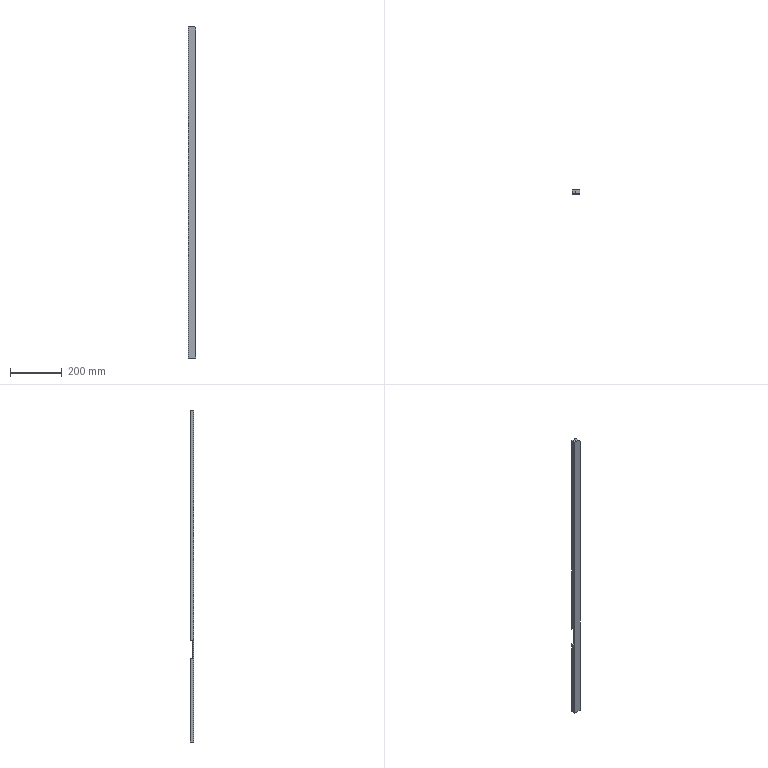Part | NX | features BREP 1 | 1 solid | 17 faces | box 30 x 15 x 1279 mm | volume 553706 mm3 | plane 16 | spline 1
STEP:
#1=CARTESIAN_POINT('',(1644.53,-675.072,490.012));
#2=VERTEX_POINT('',#1);
#3=CARTESIAN_POINT('',(1635.458,-675.072,490.012));
#4=VERTEX_POINT('',#3);
#5=CARTESIAN_POINT('',(1644.53,-675.072,490.012));
#6=CARTESIAN_POINT('',(1635.458,-675.072,490.012));
#7=B_SPLINE_CURVE_WITH_KNOTS('',1,(#5,#6),.UNSPECIFIED.,.F.,.F.,(2,2),(0.,9.072),.UNSPECIFIED.);
#8=EDGE_CURVE('',#2,#4,#7,.T.);
#9=ORIENTED_EDGE('',*,*,#8,.F.);
#10=CARTESIAN_POINT('',(1644.53,-675.072,420.012));
#11=VERTEX_POINT('',#10);
#12=CARTESIAN_POINT('',(1644.53,-675.072,455.012));
#13=DIRECTION('',(0.,0.,-1.));
#14=VECTOR('',#13,1000.);
#15=LINE('',#12,#14);
#16=EDGE_CURVE('',#2,#11,#15,.T.);
#17=ORIENTED_EDGE('',*,*,#16,.T.);
#18=CARTESIAN_POINT('',(1635.458,-675.072,420.012));
#19=VERTEX_POINT('',#18);
#20=CARTESIAN_POINT('',(1644.53,-675.072,420.012));
#21=CARTESIAN_POINT('',(1635.458,-675.072,420.012));
#22=B_SPLINE_CURVE_WITH_KNOTS('',1,(#20,#21),.UNSPECIFIED.,.F.,.F.,(2,2),(0.,9.072),.UNSPECIFIED.);
#23=EDGE_CURVE('',#11,#19,#22,.T.);
#24=ORIENTED_EDGE('',*,*,#23,.T.);
#25=CARTESIAN_POINT('',(1635.458,-675.072,455.012));
#26=DIRECTION('',(0.,0.,-1.));
#27=VECTOR('',#26,1000.);
#28=LINE('',#25,#27);
#29=EDGE_CURVE('',#4,#19,#28,.T.);
#30=ORIENTED_EDGE('',*,*,#29,.F.);
#31=EDGE_LOOP('',(#9,#17,#24,#30));
#32=FACE_BOUND('',#31,.T.);
#33=CARTESIAN_POINT('',(1639.762,-675.072,455.012));
#34=DIRECTION('',(0.,1.,0.));
#35=DIRECTION('',(-1.,0.,0.));
#36=AXIS2_PLACEMENT_3D('',#33,#34,#35);
#37=PLANE('',#36);
#38=ADVANCED_FACE('',(#32),#37,.T.);
#39=ORIENTED_EDGE('',*,*,#23,.F.);
#40=CARTESIAN_POINT('',(1644.53,-664.988,420.012));
#41=VERTEX_POINT('',#40);
#42=CARTESIAN_POINT('',(1644.53,-670.03,420.012));
#43=DIRECTION('',(0.,1.,0.));
#44=VECTOR('',#43,1000.);
#45=LINE('',#42,#44);
#46=EDGE_CURVE('',#11,#41,#45,.T.);
#47=ORIENTED_EDGE('',*,*,#46,.T.);
#48=CARTESIAN_POINT('',(1635.458,-664.988,420.012));
#49=VERTEX_POINT('',#48);
#50=CARTESIAN_POINT('',(1639.994,-664.988,420.012));
#51=DIRECTION('',(1.,0.,0.));
#52=VECTOR('',#51,1000.);
#53=LINE('',#50,#52);
#54=EDGE_CURVE('',#49,#41,#53,.T.);
#55=ORIENTED_EDGE('',*,*,#54,.F.);
#56=CARTESIAN_POINT('',(1635.458,-670.03,420.012));
#57=DIRECTION('',(0.,1.,0.));
#58=VECTOR('',#57,1000.);
#59=LINE('',#56,#58);
#60=EDGE_CURVE('',#19,#49,#59,.T.);
#61=ORIENTED_EDGE('',*,*,#60,.F.);
#62=EDGE_LOOP('',(#39,#47,#55,#61));
#63=FACE_BOUND('',#62,.T.);
#64=CARTESIAN_POINT('',(1639.762,-652.161,420.012));
#65=DIRECTION('',(0.,0.,1.));
#66=DIRECTION('',(1.,0.,0.));
#67=AXIS2_PLACEMENT_3D('',#64,#65,#66);
#68=PLANE('',#67);
#69=ADVANCED_FACE('',(#63),#68,.T.);
#70=CARTESIAN_POINT('',(1647.53,-675.072,490.012));
#71=VERTEX_POINT('',#70);
#72=CARTESIAN_POINT('',(1646.03,-675.072,490.012));
#73=DIRECTION('',(1.,0.,0.));
#74=VECTOR('',#73,1000.);
#75=LINE('',#72,#74);
#76=EDGE_CURVE('',#2,#71,#75,.T.);
#77=ORIENTED_EDGE('',*,*,#76,.T.);
#78=CARTESIAN_POINT('',(1647.53,-675.072,420.012));
#79=VERTEX_POINT('',#78);
#80=CARTESIAN_POINT('',(1647.53,-675.072,420.012));
#81=CARTESIAN_POINT('',(1647.53,-675.072,434.012));
#82=CARTESIAN_POINT('',(1647.53,-675.072,448.012));
#83=CARTESIAN_POINT('',(1647.53,-675.072,462.012));
#84=CARTESIAN_POINT('',(1647.53,-675.072,476.012));
#85=CARTESIAN_POINT('',(1647.53,-675.072,490.012));
#86=B_SPLINE_CURVE_WITH_KNOTS('',5,(#80,#81,#82,#83,#84,#85),.UNSPECIFIED.,.F.,.F.,(6,6),(0.,70.),.UNSPECIFIED.);
#87=EDGE_CURVE('',#79,#71,#86,.T.);
#88=ORIENTED_EDGE('',*,*,#87,.F.);
#89=CARTESIAN_POINT('',(1646.03,-675.072,420.012));
#90=DIRECTION('',(1.,0.,0.));
#91=VECTOR('',#90,1000.);
#92=LINE('',#89,#91);
#93=EDGE_CURVE('',#11,#79,#92,.T.);
#94=ORIENTED_EDGE('',*,*,#93,.F.);
#95=ORIENTED_EDGE('',*,*,#16,.F.);
#96=EDGE_LOOP('',(#77,#88,#94,#95));
#97=FACE_BOUND('',#96,.T.);
#98=CARTESIAN_POINT('',(1644.53,-675.072,455.012));
#99=DIRECTION('',(0.,-1.,0.));
#100=DIRECTION('',(1.,0.,0.));
#101=AXIS2_PLACEMENT_3D('',#98,#99,#100);
#102=PLANE('',#101);
#103=ADVANCED_FACE('',(#97),#102,.F.);
#104=ORIENTED_EDGE('',*,*,#46,.F.);
#105=ORIENTED_EDGE('',*,*,#93,.T.);
#106=CARTESIAN_POINT('',(1647.53,-664.988,420.012));
#107=VERTEX_POINT('',#106);
#108=CARTESIAN_POINT('',(1647.53,-664.988,420.012));
#109=CARTESIAN_POINT('',(1647.53,-667.005,420.012));
#110=CARTESIAN_POINT('',(1647.53,-669.021,420.012));
#111=CARTESIAN_POINT('',(1647.53,-671.038,420.012));
#112=CARTESIAN_POINT('',(1647.53,-673.055,420.012));
#113=CARTESIAN_POINT('',(1647.53,-675.072,420.012));
#114=B_SPLINE_CURVE_WITH_KNOTS('',5,(#108,#109,#110,#111,#112,#113),.UNSPECIFIED.,.F.,.F.,(6,6),(35.737,45.821),.UNSPECIFIED.);
#115=EDGE_CURVE('',#107,#79,#114,.T.);
#116=ORIENTED_EDGE('',*,*,#115,.F.);
#117=CARTESIAN_POINT('',(1646.03,-664.988,420.012));
#118=DIRECTION('',(1.,0.,0.));
#119=VECTOR('',#118,1000.);
#120=LINE('',#117,#119);
#121=EDGE_CURVE('',#41,#107,#120,.T.);
#122=ORIENTED_EDGE('',*,*,#121,.F.);
#123=EDGE_LOOP('',(#104,#105,#116,#122));
#124=FACE_BOUND('',#123,.T.);
#125=CARTESIAN_POINT('',(1644.53,-652.161,420.012));
#126=DIRECTION('',(0.,0.,1.));
#127=DIRECTION('',(1.,0.,0.));
#128=AXIS2_PLACEMENT_3D('',#125,#126,#127);
#129=PLANE('',#128);
#130=ADVANCED_FACE('',(#124),#129,.T.);
#131=CARTESIAN_POINT('',(1644.53,-664.988,490.012));
#132=VERTEX_POINT('',#131);
#133=CARTESIAN_POINT('',(1644.53,-670.03,490.012));
#134=DIRECTION('',(0.,-1.,0.));
#135=VECTOR('',#134,1000.);
#136=LINE('',#133,#135);
#137=EDGE_CURVE('',#132,#2,#136,.T.);
#138=ORIENTED_EDGE('',*,*,#137,.T.);
#139=ORIENTED_EDGE('',*,*,#8,.T.);
#140=CARTESIAN_POINT('',(1635.458,-664.988,490.012));
#141=VERTEX_POINT('',#140);
#142=CARTESIAN_POINT('',(1635.458,-670.03,490.012));
#143=DIRECTION('',(0.,-1.,0.));
#144=VECTOR('',#143,1000.);
#145=LINE('',#142,#144);
#146=EDGE_CURVE('',#141,#4,#145,.T.);
#147=ORIENTED_EDGE('',*,*,#146,.F.);
#148=CARTESIAN_POINT('',(1639.994,-664.988,490.012));
#149=DIRECTION('',(1.,0.,0.));
#150=VECTOR('',#149,1000.);
#151=LINE('',#148,#150);
#152=EDGE_CURVE('',#141,#132,#151,.T.);
#153=ORIENTED_EDGE('',*,*,#152,.T.);
#154=EDGE_LOOP('',(#138,#139,#147,#153));
#155=FACE_BOUND('',#154,.T.);
#156=CARTESIAN_POINT('',(1639.762,-652.161,490.012));
#157=DIRECTION('',(0.,0.,-1.));
#158=DIRECTION('',(-1.,0.,0.));
#159=AXIS2_PLACEMENT_3D('',#156,#157,#158);
#160=PLANE('',#159);
#161=ADVANCED_FACE('',(#155),#160,.T.);
#162=CARTESIAN_POINT('',(1647.53,-664.988,490.012));
#163=VERTEX_POINT('',#162);
#164=CARTESIAN_POINT('',(1646.03,-664.988,490.012));
#165=DIRECTION('',(1.,0.,0.));
#166=VECTOR('',#165,1000.);
#167=LINE('',#164,#166);
#168=EDGE_CURVE('',#132,#163,#167,.T.);
#169=ORIENTED_EDGE('',*,*,#168,.T.);
#170=CARTESIAN_POINT('',(1647.53,-675.072,490.012));
#171=CARTESIAN_POINT('',(1647.53,-673.055,490.012));
#172=CARTESIAN_POINT('',(1647.53,-671.038,490.012));
#173=CARTESIAN_POINT('',(1647.53,-669.021,490.012));
#174=CARTESIAN_POINT('',(1647.53,-667.005,490.012));
#175=CARTESIAN_POINT('',(1647.53,-664.988,490.012));
#176=B_SPLINE_CURVE_WITH_KNOTS('',5,(#170,#171,#172,#173,#174,#175),.UNSPECIFIED.,.F.,.F.,(6,6),(0.,10.084),.UNSPECIFIED.);
#177=EDGE_CURVE('',#71,#163,#176,.T.);
#178=ORIENTED_EDGE('',*,*,#177,.F.);
#179=ORIENTED_EDGE('',*,*,#76,.F.);
#180=ORIENTED_EDGE('',*,*,#137,.F.);
#181=EDGE_LOOP('',(#169,#178,#179,#180));
#182=FACE_BOUND('',#181,.T.);
#183=CARTESIAN_POINT('',(1644.53,-652.161,490.012));
#184=DIRECTION('',(0.,0.,1.));
#185=DIRECTION('',(1.,0.,0.));
#186=AXIS2_PLACEMENT_3D('',#183,#184,#185);
#187=PLANE('',#186);
#188=ADVANCED_FACE('',(#182),#187,.F.);
#189=CARTESIAN_POINT('',(1635.458,-664.988,100.));
#190=VERTEX_POINT('',#189);
#191=CARTESIAN_POINT('',(1635.458,-664.988,260.006));
#192=DIRECTION('',(0.,0.,-1.));
#193=VECTOR('',#192,1000.);
#194=LINE('',#191,#193);
#195=EDGE_CURVE('',#49,#190,#194,.T.);
#196=ORIENTED_EDGE('',*,*,#195,.T.);
#197=CARTESIAN_POINT('',(1635.458,-679.988,100.));
#198=VERTEX_POINT('',#197);
#199=CARTESIAN_POINT('',(1635.458,-672.488,100.));
#200=DIRECTION('',(0.,1.,0.));
#201=VECTOR('',#200,1000.);
#202=LINE('',#199,#201);
#203=EDGE_CURVE('',#198,#190,#202,.T.);
#204=ORIENTED_EDGE('',*,*,#203,.F.);
#205=CARTESIAN_POINT('',(1635.458,-679.988,1378.689));
#206=VERTEX_POINT('',#205);
#207=CARTESIAN_POINT('',(1635.458,-679.988,739.344));
#208=DIRECTION('',(0.,0.,-1.));
#209=VECTOR('',#208,1000.);
#210=LINE('',#207,#209);
#211=EDGE_CURVE('',#206,#198,#210,.T.);
#212=ORIENTED_EDGE('',*,*,#211,.F.);
#213=CARTESIAN_POINT('',(1635.458,-664.988,1378.689));
#214=VERTEX_POINT('',#213);
#215=CARTESIAN_POINT('',(1635.458,-672.488,1378.689));
#216=DIRECTION('',(0.,-1.,0.));
#217=VECTOR('',#216,1000.);
#218=LINE('',#215,#217);
#219=EDGE_CURVE('',#214,#206,#218,.T.);
#220=ORIENTED_EDGE('',*,*,#219,.F.);
#221=CARTESIAN_POINT('',(1635.458,-664.988,934.35));
#222=DIRECTION('',(0.,0.,-1.));
#223=VECTOR('',#222,1000.);
#224=LINE('',#221,#223);
#225=EDGE_CURVE('',#214,#141,#224,.T.);
#226=ORIENTED_EDGE('',*,*,#225,.T.);
#227=ORIENTED_EDGE('',*,*,#146,.T.);
#228=ORIENTED_EDGE('',*,*,#29,.T.);
#229=ORIENTED_EDGE('',*,*,#60,.T.);
#230=EDGE_LOOP('',(#196,#204,#212,#220,#226,#227,#228,#229));
#231=FACE_BOUND('',#230,.T.);
#232=CARTESIAN_POINT('',(1635.458,-679.988,739.344));
#233=DIRECTION('',(-1.,0.,0.));
#234=DIRECTION('',(0.,1.,0.));
#235=AXIS2_PLACEMENT_3D('',#232,#233,#234);
#236=PLANE('',#235);
#237=ADVANCED_FACE('',(#231),#236,.T.);
#238=CARTESIAN_POINT('',(1665.458,-664.988,420.012));
#239=VERTEX_POINT('',#238);
#240=CARTESIAN_POINT('',(1665.458,-664.988,100.));
#241=VERTEX_POINT('',#240);
#242=CARTESIAN_POINT('',(1665.458,-664.988,260.006));
#243=DIRECTION('',(0.,0.,-1.));
#244=VECTOR('',#243,1000.);
#245=LINE('',#242,#244);
#246=EDGE_CURVE('',#239,#241,#245,.T.);
#247=ORIENTED_EDGE('',*,*,#246,.T.);
#248=CARTESIAN_POINT('',(1650.458,-664.988,100.));
#249=DIRECTION('',(1.,0.,0.));
#250=VECTOR('',#249,1000.);
#251=LINE('',#248,#250);
#252=EDGE_CURVE('',#190,#241,#251,.T.);
#253=ORIENTED_EDGE('',*,*,#252,.F.);
#254=ORIENTED_EDGE('',*,*,#195,.F.);
#255=ORIENTED_EDGE('',*,*,#54,.T.);
#256=ORIENTED_EDGE('',*,*,#121,.T.);
#257=CARTESIAN_POINT('',(1647.53,-664.988,420.012));
#258=CARTESIAN_POINT('',(1665.458,-664.988,420.012));
#259=B_SPLINE_CURVE_WITH_KNOTS('',1,(#257,#258),.UNSPECIFIED.,.F.,.F.,(2,2),(0.,17.928),.UNSPECIFIED.);
#260=EDGE_CURVE('',#107,#239,#259,.T.);
#261=ORIENTED_EDGE('',*,*,#260,.T.);
#262=EDGE_LOOP('',(#247,#253,#254,#255,#256,#261));
#263=FACE_BOUND('',#262,.T.);
#264=CARTESIAN_POINT('',(1635.458,-664.988,-0.2896));
#265=DIRECTION('',(0.,1.,0.));
#266=DIRECTION('',(1.,0.,0.));
#267=AXIS2_PLACEMENT_3D('',#264,#265,#266);
#268=PLANE('',#267);
#269=ADVANCED_FACE('',(#263),#268,.T.);
#270=CARTESIAN_POINT('',(1665.458,-679.988,100.));
#271=VERTEX_POINT('',#270);
#272=CARTESIAN_POINT('',(1650.458,-679.988,100.));
#273=DIRECTION('',(1.,0.,0.));
#274=VECTOR('',#273,1000.);
#275=LINE('',#272,#274);
#276=EDGE_CURVE('',#198,#271,#275,.T.);
#277=ORIENTED_EDGE('',*,*,#276,.F.);
#278=ORIENTED_EDGE('',*,*,#203,.T.);
#279=ORIENTED_EDGE('',*,*,#252,.T.);
#280=CARTESIAN_POINT('',(1665.458,-672.488,100.));
#281=DIRECTION('',(0.,1.,0.));
#282=VECTOR('',#281,1000.);
#283=LINE('',#280,#282);
#284=EDGE_CURVE('',#271,#241,#283,.T.);
#285=ORIENTED_EDGE('',*,*,#284,.F.);
#286=EDGE_LOOP('',(#277,#278,#279,#285));
#287=FACE_BOUND('',#286,.T.);
#288=CARTESIAN_POINT('',(1650.458,-679.988,100.));
#289=DIRECTION('',(0.,0.,-1.));
#290=DIRECTION('',(1.,0.,0.));
#291=AXIS2_PLACEMENT_3D('',#288,#289,#290);
#292=PLANE('',#291);
#293=ADVANCED_FACE('',(#287),#292,.T.);
#294=CARTESIAN_POINT('',(1665.458,-675.072,490.012));
#295=VERTEX_POINT('',#294);
#296=CARTESIAN_POINT('',(1647.53,-675.072,490.012));
#297=CARTESIAN_POINT('',(1665.458,-675.072,490.012));
#298=B_SPLINE_CURVE_WITH_KNOTS('',1,(#296,#297),.UNSPECIFIED.,.F.,.F.,(2,2),(0.,17.928),.UNSPECIFIED.);
#299=EDGE_CURVE('',#71,#295,#298,.T.);
#300=ORIENTED_EDGE('',*,*,#299,.F.);
#301=ORIENTED_EDGE('',*,*,#177,.T.);
#302=CARTESIAN_POINT('',(1665.458,-664.988,490.012));
#303=VERTEX_POINT('',#302);
#304=CARTESIAN_POINT('',(1656.494,-664.988,490.012));
#305=DIRECTION('',(1.,0.,0.));
#306=VECTOR('',#305,1000.);
#307=LINE('',#304,#306);
#308=EDGE_CURVE('',#163,#303,#307,.T.);
#309=ORIENTED_EDGE('',*,*,#308,.T.);
#310=CARTESIAN_POINT('',(1665.458,-670.03,490.012));
#311=DIRECTION('',(0.,1.,0.));
#312=VECTOR('',#311,1000.);
#313=LINE('',#310,#312);
#314=EDGE_CURVE('',#295,#303,#313,.T.);
#315=ORIENTED_EDGE('',*,*,#314,.F.);
#316=EDGE_LOOP('',(#300,#301,#309,#315));
#317=FACE_BOUND('',#316,.T.);
#318=CARTESIAN_POINT('',(1657.1,-652.161,490.012));
#319=DIRECTION('',(0.,0.,-1.));
#320=DIRECTION('',(0.,1.,0.));
#321=AXIS2_PLACEMENT_3D('',#318,#319,#320);
#322=PLANE('',#321);
#323=ADVANCED_FACE('',(#317),#322,.T.);
#324=CARTESIAN_POINT('',(1665.458,-675.072,420.012));
#325=VERTEX_POINT('',#324);
#326=CARTESIAN_POINT('',(1647.53,-675.072,420.012));
#327=CARTESIAN_POINT('',(1665.458,-675.072,420.012));
#328=B_SPLINE_CURVE_WITH_KNOTS('',1,(#326,#327),.UNSPECIFIED.,.F.,.F.,(2,2),(0.,17.928),.UNSPECIFIED.);
#329=EDGE_CURVE('',#79,#325,#328,.T.);
#330=ORIENTED_EDGE('',*,*,#329,.F.);
#331=ORIENTED_EDGE('',*,*,#87,.T.);
#332=ORIENTED_EDGE('',*,*,#299,.T.);
#333=CARTESIAN_POINT('',(1665.458,-675.072,455.012));
#334=DIRECTION('',(0.,0.,1.));
#335=VECTOR('',#334,1000.);
#336=LINE('',#333,#335);
#337=EDGE_CURVE('',#325,#295,#336,.T.);
#338=ORIENTED_EDGE('',*,*,#337,.F.);
#339=EDGE_LOOP('',(#330,#331,#332,#338));
#340=FACE_BOUND('',#339,.T.);
#341=CARTESIAN_POINT('',(1657.1,-675.072,455.012));
#342=DIRECTION('',(0.,1.,0.));
#343=DIRECTION('',(-1.,0.,0.));
#344=AXIS2_PLACEMENT_3D('',#341,#342,#343);
#345=PLANE('',#344);
#346=ADVANCED_FACE('',(#340),#345,.T.);
#347=ORIENTED_EDGE('',*,*,#115,.T.);
#348=ORIENTED_EDGE('',*,*,#329,.T.);
#349=CARTESIAN_POINT('',(1665.458,-670.03,420.012));
#350=DIRECTION('',(0.,-1.,0.));
#351=VECTOR('',#350,1000.);
#352=LINE('',#349,#351);
#353=EDGE_CURVE('',#239,#325,#352,.T.);
#354=ORIENTED_EDGE('',*,*,#353,.F.);
#355=ORIENTED_EDGE('',*,*,#260,.F.);
#356=EDGE_LOOP('',(#347,#348,#354,#355));
#357=FACE_BOUND('',#356,.T.);
#358=CARTESIAN_POINT('',(1657.1,-652.161,420.012));
#359=DIRECTION('',(0.,0.,1.));
#360=DIRECTION('',(0.,-1.,0.));
#361=AXIS2_PLACEMENT_3D('',#358,#359,#360);
#362=PLANE('',#361);
#363=ADVANCED_FACE('',(#357),#362,.T.);
#364=CARTESIAN_POINT('',(1665.458,-679.988,1362.508));
#365=VERTEX_POINT('',#364);
#366=CARTESIAN_POINT('',(1665.458,-679.988,731.254));
#367=DIRECTION('',(0.,0.,-1.));
#368=VECTOR('',#367,1000.);
#369=LINE('',#366,#368);
#370=EDGE_CURVE('',#365,#271,#369,.T.);
#371=ORIENTED_EDGE('',*,*,#370,.F.);
#372=CARTESIAN_POINT('',(1647.785,-679.988,1378.689));
#373=VERTEX_POINT('',#372);
#374=CARTESIAN_POINT('',(1665.458,-679.988,1362.508));
#375=CARTESIAN_POINT('',(1665.444,-679.988,1364.171));
#376=CARTESIAN_POINT('',(1665.39,-679.988,1365.833));
#377=CARTESIAN_POINT('',(1665.236,-679.988,1367.467));
#378=CARTESIAN_POINT('',(1664.759,-679.988,1369.901));
#379=CARTESIAN_POINT('',(1663.774,-679.988,1372.149));
#380=CARTESIAN_POINT('',(1663.413,-679.988,1372.821));
#381=CARTESIAN_POINT('',(1662.848,-679.988,1373.687));
#382=CARTESIAN_POINT('',(1662.182,-679.988,1374.472));
#383=CARTESIAN_POINT('',(1662.021,-679.988,1374.65));
#384=CARTESIAN_POINT('',(1661.2,-679.988,1375.509));
#385=CARTESIAN_POINT('',(1660.263,-679.988,1376.249));
#386=CARTESIAN_POINT('',(1659.431,-679.988,1376.753));
#387=CARTESIAN_POINT('',(1657.06,-679.988,1377.889));
#388=CARTESIAN_POINT('',(1654.466,-679.988,1378.434));
#389=CARTESIAN_POINT('',(1652.796,-679.988,1378.606));
#390=CARTESIAN_POINT('',(1650.79,-679.988,1378.676));
#391=CARTESIAN_POINT('',(1648.783,-679.988,1378.688));
#392=CARTESIAN_POINT('',(1648.451,-679.988,1378.689));
#393=CARTESIAN_POINT('',(1648.118,-679.988,1378.689));
#394=CARTESIAN_POINT('',(1647.785,-679.988,1378.689));
#395=B_SPLINE_CURVE_WITH_KNOTS('',5,(#374,#375,#376,#377,#378,#379,#380,#381,#382,#383,#384,#385,#386,#387,#388,#389,#390,#391,#392,#393,#394),.UNSPECIFIED.,.F.,.F.,(6,3,3,3,3,3,6),(0.,8.317,12.271,13.482,18.214,26.594,28.26),.UNSPECIFIED.);
#396=EDGE_CURVE('',#365,#373,#395,.T.);
#397=ORIENTED_EDGE('',*,*,#396,.T.);
#398=CARTESIAN_POINT('',(1641.622,-679.988,1378.689));
#399=DIRECTION('',(1.,0.,0.));
#400=VECTOR('',#399,1000.);
#401=LINE('',#398,#400);
#402=EDGE_CURVE('',#206,#373,#401,.T.);
#403=ORIENTED_EDGE('',*,*,#402,.F.);
#404=ORIENTED_EDGE('',*,*,#211,.T.);
#405=ORIENTED_EDGE('',*,*,#276,.T.);
#406=EDGE_LOOP('',(#371,#397,#403,#404,#405));
#407=FACE_BOUND('',#406,.T.);
#408=CARTESIAN_POINT('',(1635.458,-679.988,-0.2896));
#409=DIRECTION('',(0.,1.,0.));
#410=DIRECTION('',(1.,0.,0.));
#411=AXIS2_PLACEMENT_3D('',#408,#409,#410);
#412=PLANE('',#411);
#413=ADVANCED_FACE('',(#407),#412,.F.);
#414=CARTESIAN_POINT('',(1647.785,-664.988,1378.689));
#415=VERTEX_POINT('',#414);
#416=CARTESIAN_POINT('',(1647.785,-679.988,1378.689));
#417=DIRECTION('',(0.,1.,0.));
#418=VECTOR('',#417,1000.);
#419=LINE('',#416,#418);
#420=EDGE_CURVE('',#373,#415,#419,.T.);
#421=ORIENTED_EDGE('',*,*,#420,.T.);
#422=CARTESIAN_POINT('',(1641.622,-664.988,1378.689));
#423=DIRECTION('',(1.,0.,0.));
#424=VECTOR('',#423,1000.);
#425=LINE('',#422,#424);
#426=EDGE_CURVE('',#214,#415,#425,.T.);
#427=ORIENTED_EDGE('',*,*,#426,.F.);
#428=ORIENTED_EDGE('',*,*,#219,.T.);
#429=ORIENTED_EDGE('',*,*,#402,.T.);
#430=EDGE_LOOP('',(#421,#427,#428,#429));
#431=FACE_BOUND('',#430,.T.);
#432=CARTESIAN_POINT('',(1641.622,-679.988,1378.689));
#433=DIRECTION('',(0.,0.,-1.));
#434=DIRECTION('',(1.,0.,0.));
#435=AXIS2_PLACEMENT_3D('',#432,#433,#434);
#436=PLANE('',#435);
#437=ADVANCED_FACE('',(#431),#436,.F.);
#438=ORIENTED_EDGE('',*,*,#225,.F.);
#439=ORIENTED_EDGE('',*,*,#426,.T.);
#440=CARTESIAN_POINT('',(1665.458,-664.988,1362.508));
#441=VERTEX_POINT('',#440);
#442=CARTESIAN_POINT('',(1665.458,-664.988,1362.508));
#443=CARTESIAN_POINT('',(1665.444,-664.988,1364.171));
#444=CARTESIAN_POINT('',(1665.39,-664.988,1365.833));
#445=CARTESIAN_POINT('',(1665.236,-664.988,1367.467));
#446=CARTESIAN_POINT('',(1664.759,-664.988,1369.901));
#447=CARTESIAN_POINT('',(1663.774,-664.988,1372.149));
#448=CARTESIAN_POINT('',(1663.413,-664.988,1372.821));
#449=CARTESIAN_POINT('',(1662.848,-664.988,1373.687));
#450=CARTESIAN_POINT('',(1662.182,-664.988,1374.472));
#451=CARTESIAN_POINT('',(1662.021,-664.988,1374.65));
#452=CARTESIAN_POINT('',(1661.2,-664.988,1375.509));
#453=CARTESIAN_POINT('',(1660.263,-664.988,1376.249));
#454=CARTESIAN_POINT('',(1659.431,-664.988,1376.753));
#455=CARTESIAN_POINT('',(1657.06,-664.988,1377.889));
#456=CARTESIAN_POINT('',(1654.466,-664.988,1378.434));
#457=CARTESIAN_POINT('',(1652.796,-664.988,1378.606));
#458=CARTESIAN_POINT('',(1650.79,-664.988,1378.676));
#459=CARTESIAN_POINT('',(1648.783,-664.988,1378.688));
#460=CARTESIAN_POINT('',(1648.451,-664.988,1378.689));
#461=CARTESIAN_POINT('',(1648.118,-664.988,1378.689));
#462=CARTESIAN_POINT('',(1647.785,-664.988,1378.689));
#463=B_SPLINE_CURVE_WITH_KNOTS('',5,(#442,#443,#444,#445,#446,#447,#448,#449,#450,#451,#452,#453,#454,#455,#456,#457,#458,#459,#460,#461,#462),.UNSPECIFIED.,.F.,.F.,(6,3,3,3,3,3,6),(0.,8.317,12.271,13.482,18.214,26.594,28.26),.UNSPECIFIED.);
#464=EDGE_CURVE('',#441,#415,#463,.T.);
#465=ORIENTED_EDGE('',*,*,#464,.F.);
#466=CARTESIAN_POINT('',(1665.458,-664.988,926.26));
#467=DIRECTION('',(0.,0.,-1.));
#468=VECTOR('',#467,1000.);
#469=LINE('',#466,#468);
#470=EDGE_CURVE('',#441,#303,#469,.T.);
#471=ORIENTED_EDGE('',*,*,#470,.T.);
#472=ORIENTED_EDGE('',*,*,#308,.F.);
#473=ORIENTED_EDGE('',*,*,#168,.F.);
#474=ORIENTED_EDGE('',*,*,#152,.F.);
#475=EDGE_LOOP('',(#438,#439,#465,#471,#472,#473,#474));
#476=FACE_BOUND('',#475,.T.);
#477=CARTESIAN_POINT('',(1635.458,-664.988,-0.2896));
#478=DIRECTION('',(0.,1.,0.));
#479=DIRECTION('',(1.,0.,0.));
#480=AXIS2_PLACEMENT_3D('',#477,#478,#479);
#481=PLANE('',#480);
#482=ADVANCED_FACE('',(#476),#481,.T.);
#483=ORIENTED_EDGE('',*,*,#353,.T.);
#484=ORIENTED_EDGE('',*,*,#337,.T.);
#485=ORIENTED_EDGE('',*,*,#314,.T.);
#486=ORIENTED_EDGE('',*,*,#470,.F.);
#487=CARTESIAN_POINT('',(1665.458,-679.988,1362.508));
#488=DIRECTION('',(0.,1.,0.));
#489=VECTOR('',#488,1000.);
#490=LINE('',#487,#489);
#491=EDGE_CURVE('',#365,#441,#490,.T.);
#492=ORIENTED_EDGE('',*,*,#491,.F.);
#493=ORIENTED_EDGE('',*,*,#370,.T.);
#494=ORIENTED_EDGE('',*,*,#284,.T.);
#495=ORIENTED_EDGE('',*,*,#246,.F.);
#496=EDGE_LOOP('',(#483,#484,#485,#486,#492,#493,#494,#495));
#497=FACE_BOUND('',#496,.T.);
#498=CARTESIAN_POINT('',(1665.458,-679.988,731.254));
#499=DIRECTION('',(-1.,0.,0.));
#500=DIRECTION('',(0.,1.,0.));
#501=AXIS2_PLACEMENT_3D('',#498,#499,#500);
#502=PLANE('',#501);
#503=ADVANCED_FACE('',(#497),#502,.F.);
#504=ORIENTED_EDGE('',*,*,#491,.T.);
#505=ORIENTED_EDGE('',*,*,#464,.T.);
#506=ORIENTED_EDGE('',*,*,#420,.F.);
#507=ORIENTED_EDGE('',*,*,#396,.F.);
#508=EDGE_LOOP('',(#504,#505,#506,#507));
#509=FACE_BOUND('',#508,.T.);
#510=CARTESIAN_POINT('',(1665.458,-679.988,1362.508));
#511=CARTESIAN_POINT('',(1665.458,-664.988,1362.508));
#512=CARTESIAN_POINT('',(1665.438,-679.988,1364.862));
#513=CARTESIAN_POINT('',(1665.438,-664.988,1364.862));
#514=CARTESIAN_POINT('',(1665.269,-679.988,1368.412));
#515=CARTESIAN_POINT('',(1665.269,-664.988,1368.412));
#516=CARTESIAN_POINT('',(1663.579,-679.988,1372.819));
#517=CARTESIAN_POINT('',(1663.579,-664.988,1372.819));
#518=CARTESIAN_POINT('',(1661.352,-679.988,1375.587));
#519=CARTESIAN_POINT('',(1661.352,-664.988,1375.587));
#520=CARTESIAN_POINT('',(1658.257,-679.988,1377.448));
#521=CARTESIAN_POINT('',(1658.257,-664.988,1377.448));
#522=CARTESIAN_POINT('',(1653.693,-679.988,1378.677));
#523=CARTESIAN_POINT('',(1653.693,-664.988,1378.677));
#524=CARTESIAN_POINT('',(1650.137,-679.988,1378.689));
#525=CARTESIAN_POINT('',(1650.137,-664.988,1378.689));
#526=CARTESIAN_POINT('',(1647.785,-679.988,1378.689));
#527=CARTESIAN_POINT('',(1647.785,-664.988,1378.689));
#528=B_SPLINE_SURFACE_WITH_KNOTS('',3,1,((#510,#511),(#512,#513),(#514,#515),(#516,#517),(#518,#519),(#520,#521),(#522,#523),(#524,#525),(#526,#527)),.SURF_OF_LINEAR_EXTRUSION.,.F.,.F.,.F.,(4,1,1,1,1,1,4),(2,2),(0.,7.065,10.597,14.13,17.662,21.195,28.26),(0.,1.),.UNSPECIFIED.);
#529=ADVANCED_FACE('',(#509),#528,.F.);
#530=CLOSED_SHELL('',(#38,#69,#103,#130,#161,#188,#237,#269,#293,#323,#346,#363,#413,#437,#482,#503,#529));
#531=MANIFOLD_SOLID_BREP('',#530);
#532=(LENGTH_UNIT()NAMED_UNIT(*)SI_UNIT(.MILLI.,.METRE.));
#533=UNCERTAINTY_MEASURE_WITH_UNIT(LENGTH_MEASURE(0.0508),#532,'','');
#534=(NAMED_UNIT(*)PLANE_ANGLE_UNIT()SI_UNIT($,.RADIAN.));
#535=(NAMED_UNIT(*)SI_UNIT($,.STERADIAN.)SOLID_ANGLE_UNIT());
#536=(GEOMETRIC_REPRESENTATION_CONTEXT(3)GLOBAL_UNCERTAINTY_ASSIGNED_CONTEXT((#533))GLOBAL_UNIT_ASSIGNED_CONTEXT((#532,#534,#535))REPRESENTATION_CONTEXT('',''));
#537=ADVANCED_BREP_SHAPE_REPRESENTATION('',(#531),#536);